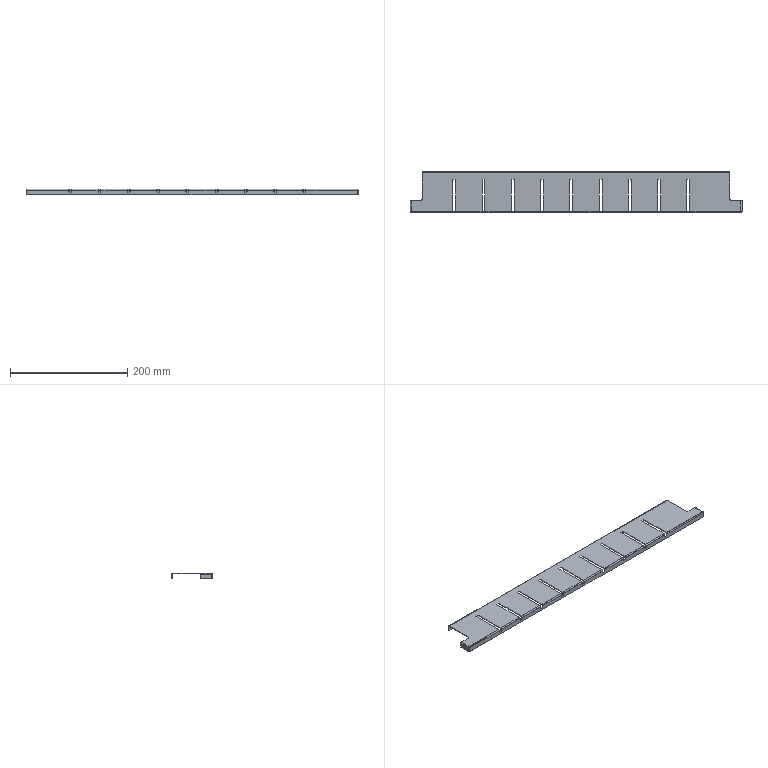Part | SolidWorks | features Cut 1, EdgeFlange 1, Fillet 1, FlatPattern 1, Fold 1, ICE 1, SMBaseFlange 1, SheetMetal 1, UnFold 1 | 1 solid | 162 faces | box 567 x 70 x 10 mm | volume 44370 mm3 | plane 94 | cylinder 64 | spline 4 | commonest cylinder face diameters 1.686 x36 4 x15 2 x13